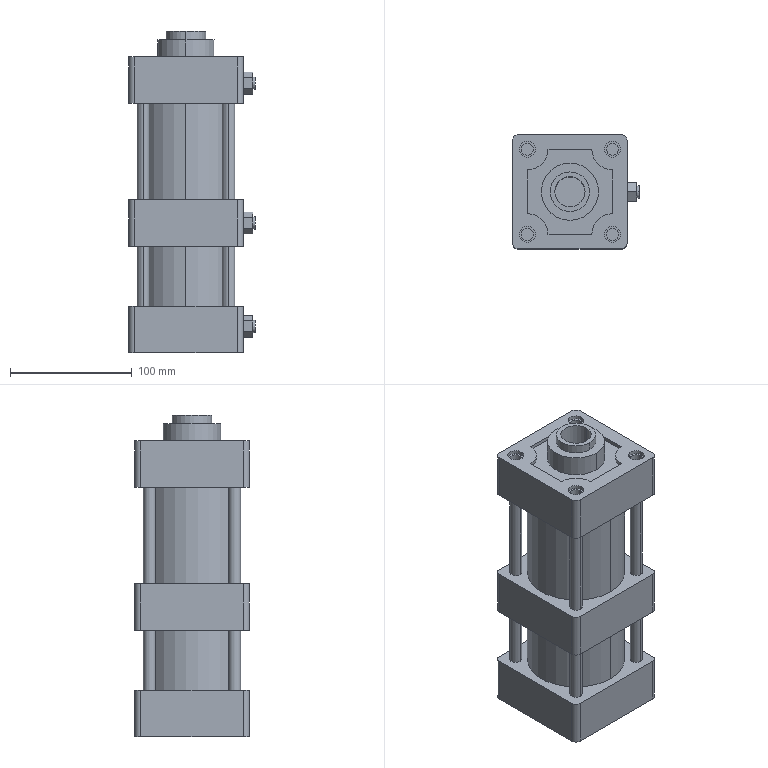Part | SolidWorks | features ICE 9, Fillet 1, Revolution 1 | 1 solid | 131 faces | box 104 x 94 x 264 mm | volume 1602001 mm3 | cylinder 70 | plane 61 | commonest cylinder face diameters 10 x30 9.4 x12 13 x8 15.806 x6 33.941 x4 80 x4